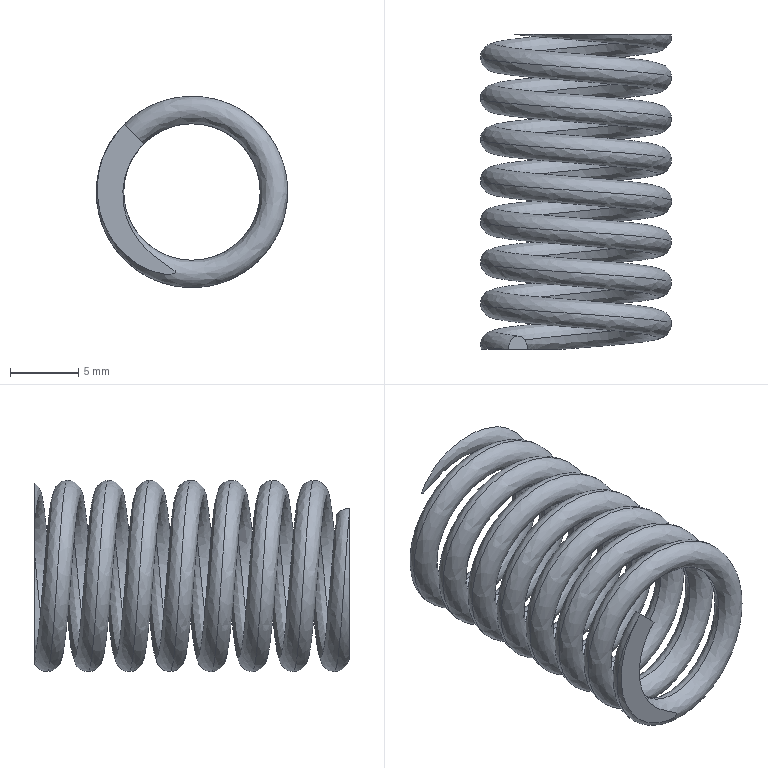Part | SolidWorks | features Helix 1, ICE 1, RefAxis 1, Sweep 1 | 1 solid | 5 faces | box 13.98 x 23 x 13.98 mm | volume 890.57 mm3 | plane 3 | spline 2